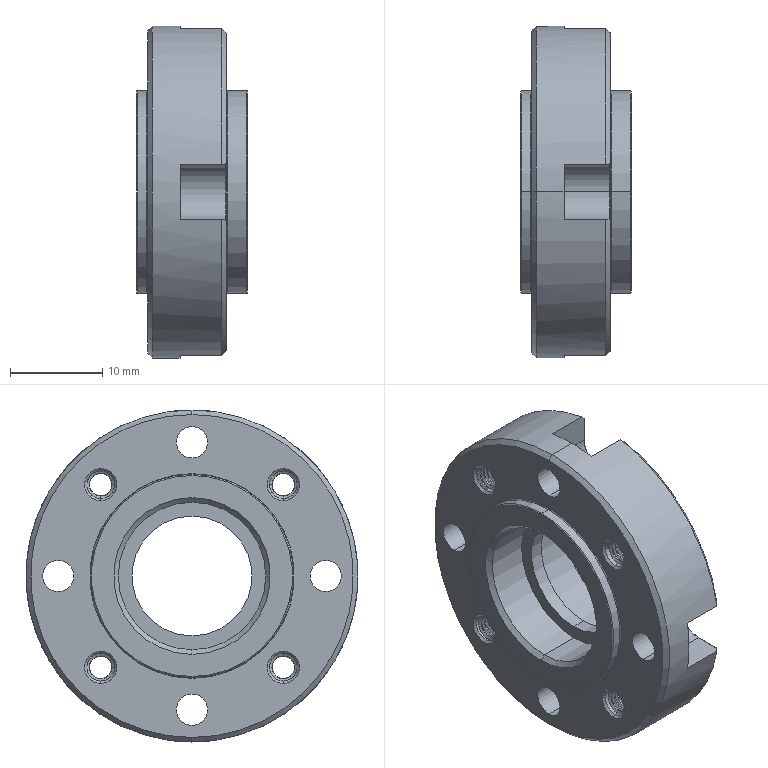Part | SolidWorks | features BaseBody 1 | 1 solid | 232 faces | box 12 x 36 x 36 mm | volume 6610 mm3 | cylinder 155 | plane 26 | cone 26 | torus 13 | spline 12 | commonest cylinder face diameters 3 x122 0.2 x8 3.4 x8 6 x5 16 x4 22 x4